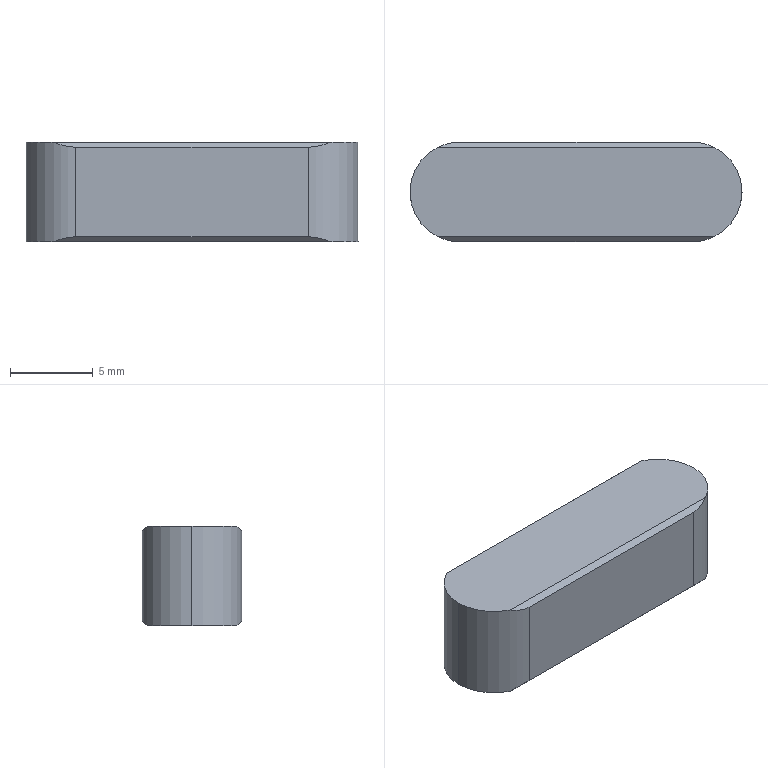Part | SolidWorks | features Extrusion 1, ICE 1 | 1 solid | 11 faces | box 20 x 6 x 6 mm | volume 670.871 mm3 | plane 8 | cylinder 3 | commonest cylinder face diameters 6 x3
STEP:
#1=CARTESIAN_POINT('',(0.,3.,6.));
#2=VERTEX_POINT('',#1);
#3=CARTESIAN_POINT('',(1.692,0.3,6.));
#4=VERTEX_POINT('',#3);
#5=CARTESIAN_POINT('',(3.,3.,6.));
#6=DIRECTION('',(0.,0.,1.));
#7=DIRECTION('',(1.,0.,0.));
#8=AXIS2_PLACEMENT_3D('',#5,#6,#7);
#9=CIRCLE('',#8,3.);
#10=EDGE_CURVE('',#2,#4,#9,.T.);
#11=ORIENTED_EDGE('',*,*,#10,.F.);
#12=CARTESIAN_POINT('',(0.,3.,0.));
#13=VERTEX_POINT('',#12);
#14=CARTESIAN_POINT('',(0.,3.,6.));
#15=DIRECTION('',(0.,0.,-1.));
#16=VECTOR('',#15,1000.);
#17=LINE('',#14,#16);
#18=EDGE_CURVE('',#2,#13,#17,.T.);
#19=ORIENTED_EDGE('',*,*,#18,.T.);
#20=CARTESIAN_POINT('',(1.692,0.3,0.));
#21=VERTEX_POINT('',#20);
#22=CARTESIAN_POINT('',(3.,3.,0.));
#23=DIRECTION('',(0.,0.,1.));
#24=DIRECTION('',(1.,0.,0.));
#25=AXIS2_PLACEMENT_3D('',#22,#23,#24);
#26=CIRCLE('',#25,3.);
#27=EDGE_CURVE('',#13,#21,#26,.T.);
#28=ORIENTED_EDGE('',*,*,#27,.T.);
#29=CARTESIAN_POINT('',(3.,0.,0.3));
#30=VERTEX_POINT('',#29);
#31=CARTESIAN_POINT('',(1.692,0.3,0.));
#32=CARTESIAN_POINT('',(2.102,0.1017,0.1983));
#33=CARTESIAN_POINT('',(2.545,0.,0.3));
#34=CARTESIAN_POINT('',(3.,0.,0.3));
#35=(BOUNDED_CURVE()B_SPLINE_CURVE(3,(#31,#32,#33,#34),.UNSPECIFIED.,.F.,.F.)B_SPLINE_CURVE_WITH_KNOTS((4,4),(2.691,3.142),.UNSPECIFIED.)CURVE()GEOMETRIC_REPRESENTATION_ITEM()RATIONAL_B_SPLINE_CURVE((1.,0.9831,0.9831,1.))REPRESENTATION_ITEM(''));
#36=EDGE_CURVE('',#21,#30,#35,.T.);
#37=ORIENTED_EDGE('',*,*,#36,.T.);
#38=CARTESIAN_POINT('',(3.,0.,5.7));
#39=VERTEX_POINT('',#38);
#40=CARTESIAN_POINT('',(3.,0.,6.));
#41=DIRECTION('',(0.,0.,-1.));
#42=VECTOR('',#41,1000.);
#43=LINE('',#40,#42);
#44=EDGE_CURVE('',#39,#30,#43,.T.);
#45=ORIENTED_EDGE('',*,*,#44,.F.);
#46=CARTESIAN_POINT('',(3.,0.,5.7));
#47=CARTESIAN_POINT('',(2.545,0.,5.7));
#48=CARTESIAN_POINT('',(2.102,0.1017,5.802));
#49=CARTESIAN_POINT('',(1.692,0.3,6.));
#50=(BOUNDED_CURVE()B_SPLINE_CURVE(3,(#46,#47,#48,#49),.UNSPECIFIED.,.F.,.F.)B_SPLINE_CURVE_WITH_KNOTS((4,4),(0.,0.451),.UNSPECIFIED.)CURVE()GEOMETRIC_REPRESENTATION_ITEM()RATIONAL_B_SPLINE_CURVE((1.,0.9831,0.9831,1.))REPRESENTATION_ITEM(''));
#51=EDGE_CURVE('',#39,#4,#50,.T.);
#52=ORIENTED_EDGE('',*,*,#51,.T.);
#53=EDGE_LOOP('',(#11,#19,#28,#37,#45,#52));
#54=FACE_OUTER_BOUND('',#53,.T.);
#55=CARTESIAN_POINT('',(3.,3.,6.));
#56=DIRECTION('',(0.,0.,-1.));
#57=DIRECTION('',(-1.,0.,0.));
#58=AXIS2_PLACEMENT_3D('',#55,#56,#57);
#59=CYLINDRICAL_SURFACE('',#58,3.);
#60=ADVANCED_FACE('',(#54),#59,.T.);
#61=ORIENTED_EDGE('',*,*,#18,.F.);
#62=CARTESIAN_POINT('',(1.692,5.7,6.));
#63=VERTEX_POINT('',#62);
#64=CARTESIAN_POINT('',(3.,3.,6.));
#65=DIRECTION('',(0.,0.,1.));
#66=DIRECTION('',(1.,0.,0.));
#67=AXIS2_PLACEMENT_3D('',#64,#65,#66);
#68=CIRCLE('',#67,3.);
#69=EDGE_CURVE('',#63,#2,#68,.T.);
#70=ORIENTED_EDGE('',*,*,#69,.F.);
#71=CARTESIAN_POINT('',(3.,6.,5.7));
#72=VERTEX_POINT('',#71);
#73=CARTESIAN_POINT('',(1.692,5.7,6.));
#74=CARTESIAN_POINT('',(2.102,5.898,5.802));
#75=CARTESIAN_POINT('',(2.545,6.,5.7));
#76=CARTESIAN_POINT('',(3.,6.,5.7));
#77=(BOUNDED_CURVE()B_SPLINE_CURVE(3,(#73,#74,#75,#76),.UNSPECIFIED.,.F.,.F.)B_SPLINE_CURVE_WITH_KNOTS((4,4),(5.832,6.283),.UNSPECIFIED.)CURVE()GEOMETRIC_REPRESENTATION_ITEM()RATIONAL_B_SPLINE_CURVE((1.,0.9831,0.9831,1.))REPRESENTATION_ITEM(''));
#78=EDGE_CURVE('',#63,#72,#77,.T.);
#79=ORIENTED_EDGE('',*,*,#78,.T.);
#80=CARTESIAN_POINT('',(3.,6.,0.3));
#81=VERTEX_POINT('',#80);
#82=CARTESIAN_POINT('',(3.,6.,6.));
#83=DIRECTION('',(0.,0.,-1.));
#84=VECTOR('',#83,1000.);
#85=LINE('',#82,#84);
#86=EDGE_CURVE('',#72,#81,#85,.T.);
#87=ORIENTED_EDGE('',*,*,#86,.T.);
#88=CARTESIAN_POINT('',(1.692,5.7,0.));
#89=VERTEX_POINT('',#88);
#90=CARTESIAN_POINT('',(3.,6.,0.3));
#91=CARTESIAN_POINT('',(2.545,6.,0.3));
#92=CARTESIAN_POINT('',(2.102,5.898,0.1983));
#93=CARTESIAN_POINT('',(1.692,5.7,0.));
#94=(BOUNDED_CURVE()B_SPLINE_CURVE(3,(#90,#91,#92,#93),.UNSPECIFIED.,.F.,.F.)B_SPLINE_CURVE_WITH_KNOTS((4,4),(3.142,3.593),.UNSPECIFIED.)CURVE()GEOMETRIC_REPRESENTATION_ITEM()RATIONAL_B_SPLINE_CURVE((1.,0.9831,0.9831,1.))REPRESENTATION_ITEM(''));
#95=EDGE_CURVE('',#81,#89,#94,.T.);
#96=ORIENTED_EDGE('',*,*,#95,.T.);
#97=CARTESIAN_POINT('',(3.,3.,0.));
#98=DIRECTION('',(0.,0.,1.));
#99=DIRECTION('',(1.,0.,0.));
#100=AXIS2_PLACEMENT_3D('',#97,#98,#99);
#101=CIRCLE('',#100,3.);
#102=EDGE_CURVE('',#89,#13,#101,.T.);
#103=ORIENTED_EDGE('',*,*,#102,.T.);
#104=EDGE_LOOP('',(#61,#70,#79,#87,#96,#103));
#105=FACE_OUTER_BOUND('',#104,.T.);
#106=CARTESIAN_POINT('',(3.,3.,6.));
#107=DIRECTION('',(0.,0.,-1.));
#108=DIRECTION('',(-1.,0.,0.));
#109=AXIS2_PLACEMENT_3D('',#106,#107,#108);
#110=CYLINDRICAL_SURFACE('',#109,3.);
#111=ADVANCED_FACE('',(#105),#110,.T.);
#112=CARTESIAN_POINT('',(17.,0.,5.7));
#113=VERTEX_POINT('',#112);
#114=CARTESIAN_POINT('',(17.,0.,0.3));
#115=VERTEX_POINT('',#114);
#116=CARTESIAN_POINT('',(17.,0.,6.));
#117=DIRECTION('',(0.,0.,-1.));
#118=VECTOR('',#117,1000.);
#119=LINE('',#116,#118);
#120=EDGE_CURVE('',#113,#115,#119,.T.);
#121=ORIENTED_EDGE('',*,*,#120,.F.);
#122=CARTESIAN_POINT('',(20.,0.,5.7));
#123=DIRECTION('',(-1.,0.,0.));
#124=VECTOR('',#123,1000.);
#125=LINE('',#122,#124);
#126=EDGE_CURVE('',#113,#39,#125,.T.);
#127=ORIENTED_EDGE('',*,*,#126,.T.);
#128=ORIENTED_EDGE('',*,*,#44,.T.);
#129=CARTESIAN_POINT('',(20.,0.,0.3));
#130=DIRECTION('',(-1.,0.,0.));
#131=VECTOR('',#130,1000.);
#132=LINE('',#129,#131);
#133=EDGE_CURVE('',#115,#30,#132,.T.);
#134=ORIENTED_EDGE('',*,*,#133,.F.);
#135=EDGE_LOOP('',(#121,#127,#128,#134));
#136=FACE_OUTER_BOUND('',#135,.T.);
#137=CARTESIAN_POINT('',(3.,0.,6.));
#138=DIRECTION('',(0.,1.,0.));
#139=DIRECTION('',(0.,0.,1.));
#140=AXIS2_PLACEMENT_3D('',#137,#138,#139);
#141=PLANE('',#140);
#142=ADVANCED_FACE('',(#136),#141,.F.);
#143=CARTESIAN_POINT('',(17.,6.,5.7));
#144=VERTEX_POINT('',#143);
#145=CARTESIAN_POINT('',(17.,6.,0.3));
#146=VERTEX_POINT('',#145);
#147=CARTESIAN_POINT('',(17.,6.,6.));
#148=DIRECTION('',(0.,0.,-1.));
#149=VECTOR('',#148,1000.);
#150=LINE('',#147,#149);
#151=EDGE_CURVE('',#144,#146,#150,.T.);
#152=ORIENTED_EDGE('',*,*,#151,.F.);
#153=CARTESIAN_POINT('',(18.308,5.7,6.));
#154=VERTEX_POINT('',#153);
#155=CARTESIAN_POINT('',(17.,6.,5.7));
#156=CARTESIAN_POINT('',(17.455,6.,5.7));
#157=CARTESIAN_POINT('',(17.898,5.898,5.802));
#158=CARTESIAN_POINT('',(18.308,5.7,6.));
#159=(BOUNDED_CURVE()B_SPLINE_CURVE(3,(#155,#156,#157,#158),.UNSPECIFIED.,.F.,.F.)B_SPLINE_CURVE_WITH_KNOTS((4,4),(0.,0.451),.UNSPECIFIED.)CURVE()GEOMETRIC_REPRESENTATION_ITEM()RATIONAL_B_SPLINE_CURVE((1.,0.9831,0.9831,1.))REPRESENTATION_ITEM(''));
#160=EDGE_CURVE('',#144,#154,#159,.T.);
#161=ORIENTED_EDGE('',*,*,#160,.T.);
#162=CARTESIAN_POINT('',(18.308,0.3,6.));
#163=VERTEX_POINT('',#162);
#164=CARTESIAN_POINT('',(17.,3.,6.));
#165=DIRECTION('',(0.,0.,1.));
#166=DIRECTION('',(1.,0.,0.));
#167=AXIS2_PLACEMENT_3D('',#164,#165,#166);
#168=CIRCLE('',#167,3.);
#169=EDGE_CURVE('',#163,#154,#168,.T.);
#170=ORIENTED_EDGE('',*,*,#169,.F.);
#171=CARTESIAN_POINT('',(18.308,0.3,6.));
#172=CARTESIAN_POINT('',(17.898,0.1017,5.802));
#173=CARTESIAN_POINT('',(17.455,0.,5.7));
#174=CARTESIAN_POINT('',(17.,0.,5.7));
#175=(BOUNDED_CURVE()B_SPLINE_CURVE(3,(#171,#172,#173,#174),.UNSPECIFIED.,.F.,.F.)B_SPLINE_CURVE_WITH_KNOTS((4,4),(5.832,6.283),.UNSPECIFIED.)CURVE()GEOMETRIC_REPRESENTATION_ITEM()RATIONAL_B_SPLINE_CURVE((1.,0.9831,0.9831,1.))REPRESENTATION_ITEM(''));
#176=EDGE_CURVE('',#163,#113,#175,.T.);
#177=ORIENTED_EDGE('',*,*,#176,.T.);
#178=ORIENTED_EDGE('',*,*,#120,.T.);
#179=CARTESIAN_POINT('',(18.308,0.3,0.));
#180=VERTEX_POINT('',#179);
#181=CARTESIAN_POINT('',(17.,0.,0.3));
#182=CARTESIAN_POINT('',(17.455,0.,0.3));
#183=CARTESIAN_POINT('',(17.898,0.1017,0.1983));
#184=CARTESIAN_POINT('',(18.308,0.3,0.));
#185=(BOUNDED_CURVE()B_SPLINE_CURVE(3,(#181,#182,#183,#184),.UNSPECIFIED.,.F.,.F.)B_SPLINE_CURVE_WITH_KNOTS((4,4),(3.142,3.593),.UNSPECIFIED.)CURVE()GEOMETRIC_REPRESENTATION_ITEM()RATIONAL_B_SPLINE_CURVE((1.,0.9831,0.9831,1.))REPRESENTATION_ITEM(''));
#186=EDGE_CURVE('',#115,#180,#185,.T.);
#187=ORIENTED_EDGE('',*,*,#186,.T.);
#188=CARTESIAN_POINT('',(18.308,5.7,0.));
#189=VERTEX_POINT('',#188);
#190=CARTESIAN_POINT('',(17.,3.,0.));
#191=DIRECTION('',(0.,0.,1.));
#192=DIRECTION('',(1.,0.,0.));
#193=AXIS2_PLACEMENT_3D('',#190,#191,#192);
#194=CIRCLE('',#193,3.);
#195=EDGE_CURVE('',#180,#189,#194,.T.);
#196=ORIENTED_EDGE('',*,*,#195,.T.);
#197=CARTESIAN_POINT('',(18.308,5.7,0.));
#198=CARTESIAN_POINT('',(17.898,5.898,0.1983));
#199=CARTESIAN_POINT('',(17.455,6.,0.3));
#200=CARTESIAN_POINT('',(17.,6.,0.3));
#201=(BOUNDED_CURVE()B_SPLINE_CURVE(3,(#197,#198,#199,#200),.UNSPECIFIED.,.F.,.T.)B_SPLINE_CURVE_WITH_KNOTS((4,4),(2.691,3.142),.UNSPECIFIED.)CURVE()GEOMETRIC_REPRESENTATION_ITEM()RATIONAL_B_SPLINE_CURVE((1.,0.9831,0.9831,1.))REPRESENTATION_ITEM(''));
#202=EDGE_CURVE('',#189,#146,#201,.T.);
#203=ORIENTED_EDGE('',*,*,#202,.T.);
#204=EDGE_LOOP('',(#152,#161,#170,#177,#178,#187,#196,#203));
#205=FACE_OUTER_BOUND('',#204,.T.);
#206=CARTESIAN_POINT('',(17.,3.,6.));
#207=DIRECTION('',(0.,0.,-1.));
#208=DIRECTION('',(-1.,0.,0.));
#209=AXIS2_PLACEMENT_3D('',#206,#207,#208);
#210=CYLINDRICAL_SURFACE('',#209,3.);
#211=ADVANCED_FACE('',(#205),#210,.T.);
#212=ORIENTED_EDGE('',*,*,#86,.F.);
#213=CARTESIAN_POINT('',(20.,6.,5.7));
#214=DIRECTION('',(-1.,0.,0.));
#215=VECTOR('',#214,1000.);
#216=LINE('',#213,#215);
#217=EDGE_CURVE('',#144,#72,#216,.T.);
#218=ORIENTED_EDGE('',*,*,#217,.F.);
#219=ORIENTED_EDGE('',*,*,#151,.T.);
#220=CARTESIAN_POINT('',(20.,6.,0.3));
#221=DIRECTION('',(-1.,0.,0.));
#222=VECTOR('',#221,1000.);
#223=LINE('',#220,#222);
#224=EDGE_CURVE('',#146,#81,#223,.T.);
#225=ORIENTED_EDGE('',*,*,#224,.T.);
#226=EDGE_LOOP('',(#212,#218,#219,#225));
#227=FACE_OUTER_BOUND('',#226,.T.);
#228=CARTESIAN_POINT('',(17.,6.,6.));
#229=DIRECTION('',(0.,-1.,0.));
#230=DIRECTION('',(0.,0.,-1.));
#231=AXIS2_PLACEMENT_3D('',#228,#229,#230);
#232=PLANE('',#231);
#233=ADVANCED_FACE('',(#227),#232,.F.);
#234=CARTESIAN_POINT('',(3.,5.7,6.));
#235=DIRECTION('',(1.,0.,0.));
#236=VECTOR('',#235,1000.);
#237=LINE('',#234,#236);
#238=EDGE_CURVE('',#63,#154,#237,.T.);
#239=ORIENTED_EDGE('',*,*,#238,.F.);
#240=ORIENTED_EDGE('',*,*,#69,.T.);
#241=ORIENTED_EDGE('',*,*,#10,.T.);
#242=CARTESIAN_POINT('',(3.,0.3,6.));
#243=DIRECTION('',(-1.,0.,0.));
#244=VECTOR('',#243,1000.);
#245=LINE('',#242,#244);
#246=EDGE_CURVE('',#163,#4,#245,.T.);
#247=ORIENTED_EDGE('',*,*,#246,.F.);
#248=ORIENTED_EDGE('',*,*,#169,.T.);
#249=EDGE_LOOP('',(#239,#240,#241,#247,#248));
#250=FACE_OUTER_BOUND('',#249,.T.);
#251=CARTESIAN_POINT('',(3.,3.,6.));
#252=DIRECTION('',(0.,0.,1.));
#253=DIRECTION('',(1.,0.,0.));
#254=AXIS2_PLACEMENT_3D('',#251,#252,#253);
#255=PLANE('',#254);
#256=ADVANCED_FACE('',(#250),#255,.T.);
#257=ORIENTED_EDGE('',*,*,#195,.F.);
#258=CARTESIAN_POINT('',(3.,0.3,0.));
#259=DIRECTION('',(-1.,0.,0.));
#260=VECTOR('',#259,1000.);
#261=LINE('',#258,#260);
#262=EDGE_CURVE('',#180,#21,#261,.T.);
#263=ORIENTED_EDGE('',*,*,#262,.T.);
#264=ORIENTED_EDGE('',*,*,#27,.F.);
#265=ORIENTED_EDGE('',*,*,#102,.F.);
#266=CARTESIAN_POINT('',(3.,5.7,0.));
#267=DIRECTION('',(1.,0.,0.));
#268=VECTOR('',#267,1000.);
#269=LINE('',#266,#268);
#270=EDGE_CURVE('',#89,#189,#269,.T.);
#271=ORIENTED_EDGE('',*,*,#270,.T.);
#272=EDGE_LOOP('',(#257,#263,#264,#265,#271));
#273=FACE_OUTER_BOUND('',#272,.T.);
#274=CARTESIAN_POINT('',(3.,3.,0.));
#275=DIRECTION('',(0.,0.,1.));
#276=DIRECTION('',(1.,0.,0.));
#277=AXIS2_PLACEMENT_3D('',#274,#275,#276);
#278=PLANE('',#277);
#279=ADVANCED_FACE('',(#273),#278,.F.);
#280=ORIENTED_EDGE('',*,*,#224,.F.);
#281=ORIENTED_EDGE('',*,*,#202,.F.);
#282=ORIENTED_EDGE('',*,*,#270,.F.);
#283=ORIENTED_EDGE('',*,*,#95,.F.);
#284=EDGE_LOOP('',(#280,#281,#282,#283));
#285=FACE_OUTER_BOUND('',#284,.T.);
#286=CARTESIAN_POINT('',(20.,5.7,0.));
#287=DIRECTION('',(0.,-0.7071,0.7071));
#288=DIRECTION('',(0.,-0.7071,-0.7071));
#289=AXIS2_PLACEMENT_3D('',#286,#287,#288);
#290=PLANE('',#289);
#291=ADVANCED_FACE('',(#285),#290,.F.);
#292=ORIENTED_EDGE('',*,*,#262,.F.);
#293=ORIENTED_EDGE('',*,*,#186,.F.);
#294=ORIENTED_EDGE('',*,*,#133,.T.);
#295=ORIENTED_EDGE('',*,*,#36,.F.);
#296=EDGE_LOOP('',(#292,#293,#294,#295));
#297=FACE_OUTER_BOUND('',#296,.T.);
#298=CARTESIAN_POINT('',(20.,0.,0.3));
#299=DIRECTION('',(0.,0.7071,0.7071));
#300=DIRECTION('',(0.,-0.7071,0.7071));
#301=AXIS2_PLACEMENT_3D('',#298,#299,#300);
#302=PLANE('',#301);
#303=ADVANCED_FACE('',(#297),#302,.F.);
#304=ORIENTED_EDGE('',*,*,#126,.F.);
#305=ORIENTED_EDGE('',*,*,#176,.F.);
#306=ORIENTED_EDGE('',*,*,#246,.T.);
#307=ORIENTED_EDGE('',*,*,#51,.F.);
#308=EDGE_LOOP('',(#304,#305,#306,#307));
#309=FACE_OUTER_BOUND('',#308,.T.);
#310=CARTESIAN_POINT('',(20.,0.3,6.));
#311=DIRECTION('',(0.,0.7071,-0.7071));
#312=DIRECTION('',(0.,0.7071,0.7071));
#313=AXIS2_PLACEMENT_3D('',#310,#311,#312);
#314=PLANE('',#313);
#315=ADVANCED_FACE('',(#309),#314,.F.);
#316=ORIENTED_EDGE('',*,*,#238,.T.);
#317=ORIENTED_EDGE('',*,*,#160,.F.);
#318=ORIENTED_EDGE('',*,*,#217,.T.);
#319=ORIENTED_EDGE('',*,*,#78,.F.);
#320=EDGE_LOOP('',(#316,#317,#318,#319));
#321=FACE_OUTER_BOUND('',#320,.T.);
#322=CARTESIAN_POINT('',(20.,6.,5.7));
#323=DIRECTION('',(0.,-0.7071,-0.7071));
#324=DIRECTION('',(0.,0.7071,-0.7071));
#325=AXIS2_PLACEMENT_3D('',#322,#323,#324);
#326=PLANE('',#325);
#327=ADVANCED_FACE('',(#321),#326,.F.);
#328=CLOSED_SHELL('',(#60,#111,#142,#211,#233,#256,#279,#291,#303,#315,#327));
#329=MANIFOLD_SOLID_BREP('',#328);
#330=CARTESIAN_POINT('',(0.,0.,0.));
#331=DIRECTION('',(0.,0.,1.));
#332=DIRECTION('',(1.,0.,0.));
#333=AXIS2_PLACEMENT_3D('',#330,#331,#332);
#334=(LENGTH_UNIT()NAMED_UNIT(*)SI_UNIT(.MILLI.,.METRE.));
#335=UNCERTAINTY_MEASURE_WITH_UNIT(LENGTH_MEASURE(0.00001),#334,'','');
#336=(NAMED_UNIT(*)PLANE_ANGLE_UNIT()SI_UNIT($,.RADIAN.));
#337=(NAMED_UNIT(*)SI_UNIT($,.STERADIAN.)SOLID_ANGLE_UNIT());
#338=(GEOMETRIC_REPRESENTATION_CONTEXT(3)GLOBAL_UNCERTAINTY_ASSIGNED_CONTEXT((#335))GLOBAL_UNIT_ASSIGNED_CONTEXT((#334,#336,#337))REPRESENTATION_CONTEXT('',''));
#339=ADVANCED_BREP_SHAPE_REPRESENTATION('',(#329,#333),#338);